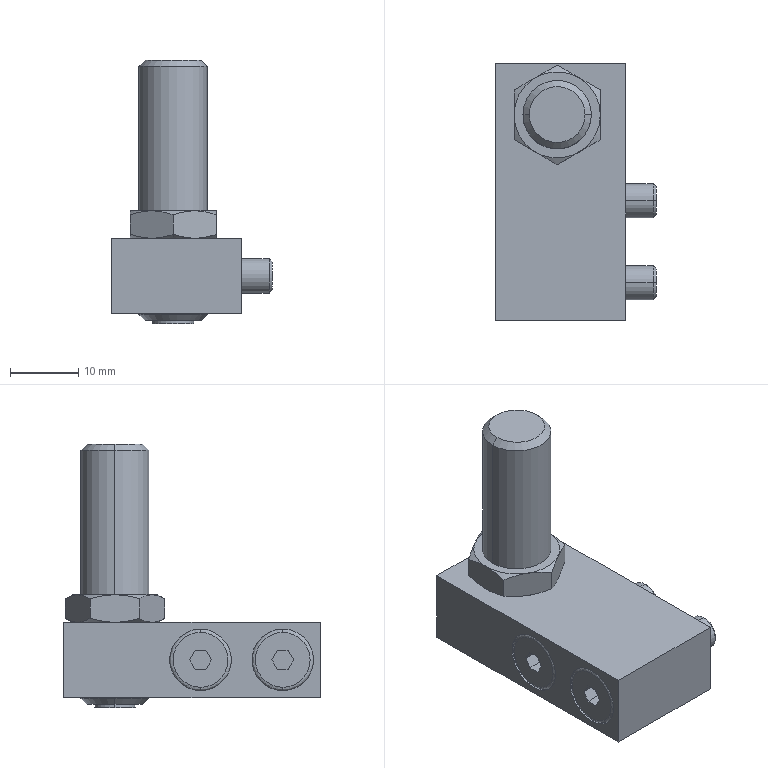Part | SolidWorks | features BaseBody 1 | 1 solid | 64 faces | box 23.5 x 37.5 x 38.5 mm | volume 10323 mm3 | plane 34 | cylinder 14 | cone 12 | spline 4 | commonest cylinder face diameters 5 x4 9 x4 10 x4 6 x2